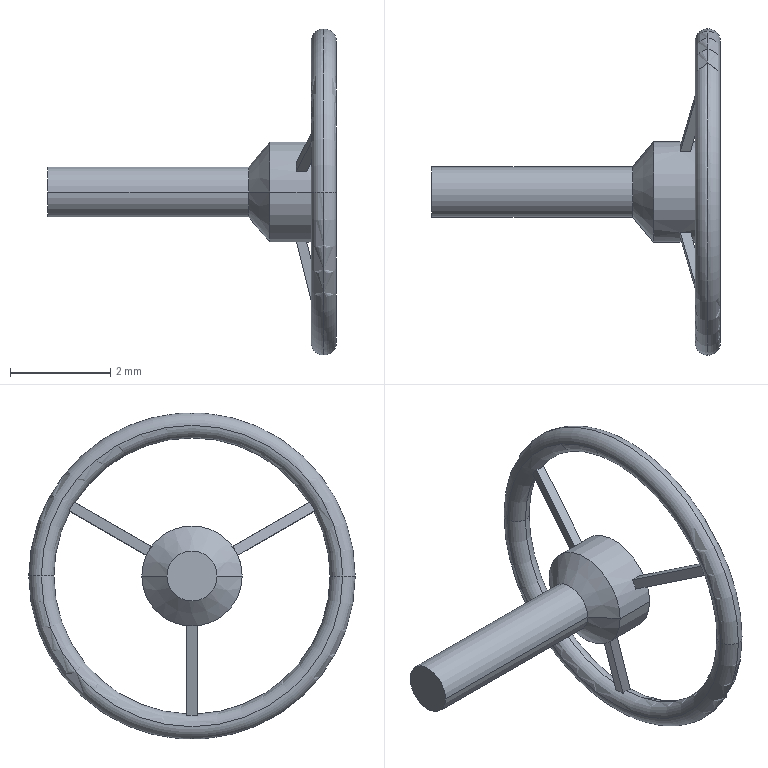Part | SolidWorks | features ICE 2, CirPattern 1, Fillet 1, Revolution 1 | 1 solid | 35 faces | box 5.75 x 6.5 x 6.5 mm | volume 10.173 mm3 | plane 19 | torus 8 | cylinder 4 | cone 4 | commonest cylinder face diameters 1 x2 2 x2
STEP:
#1=CARTESIAN_POINT('',(5.75,3.,0.));
#2=VERTEX_POINT('',#1);
#3=CARTESIAN_POINT('',(5.75,-3.,0.));
#4=VERTEX_POINT('',#3);
#5=CARTESIAN_POINT('',(5.75,0.,0.));
#6=DIRECTION('',(1.,0.,0.));
#7=DIRECTION('',(0.,-1.,0.));
#8=AXIS2_PLACEMENT_3D('',#5,#6,#7);
#9=CIRCLE('',#8,3.);
#10=EDGE_CURVE('',#2,#4,#9,.T.);
#11=ORIENTED_EDGE('',*,*,#10,.F.);
#12=CARTESIAN_POINT('',(5.5,3.25,0.));
#13=VERTEX_POINT('',#12);
#14=CARTESIAN_POINT('',(5.5,3.,0.));
#15=DIRECTION('',(0.,0.,1.));
#16=DIRECTION('',(0.,-1.,0.));
#17=AXIS2_PLACEMENT_3D('',#14,#15,#16);
#18=CIRCLE('',#17,0.25);
#19=EDGE_CURVE('',#2,#13,#18,.T.);
#20=ORIENTED_EDGE('',*,*,#19,.T.);
#21=CARTESIAN_POINT('',(5.5,-3.25,0.));
#22=VERTEX_POINT('',#21);
#23=CARTESIAN_POINT('',(5.5,0.,0.));
#24=DIRECTION('',(1.,0.,0.));
#25=DIRECTION('',(0.,-1.,0.));
#26=AXIS2_PLACEMENT_3D('',#23,#24,#25);
#27=CIRCLE('',#26,3.25);
#28=EDGE_CURVE('',#13,#22,#27,.T.);
#29=ORIENTED_EDGE('',*,*,#28,.T.);
#30=CARTESIAN_POINT('',(5.5,-3.,0.));
#31=DIRECTION('',(0.,0.,-1.));
#32=DIRECTION('',(-1.,0.,0.));
#33=AXIS2_PLACEMENT_3D('',#30,#31,#32);
#34=CIRCLE('',#33,0.25);
#35=EDGE_CURVE('',#4,#22,#34,.T.);
#36=ORIENTED_EDGE('',*,*,#35,.F.);
#37=EDGE_LOOP('',(#11,#20,#29,#36));
#38=FACE_OUTER_BOUND('',#37,.T.);
#39=CARTESIAN_POINT('',(5.5,0.,0.));
#40=DIRECTION('',(-1.,0.,0.));
#41=DIRECTION('',(0.,-1.,0.));
#42=AXIS2_PLACEMENT_3D('',#39,#40,#41);
#43=TOROIDAL_SURFACE('',#42,3.,0.25);
#44=ADVANCED_FACE('',(#38),#43,.T.);
#45=ORIENTED_EDGE('',*,*,#28,.F.);
#46=CARTESIAN_POINT('',(5.25,3.,0.));
#47=VERTEX_POINT('',#46);
#48=CARTESIAN_POINT('',(5.5,3.,0.));
#49=DIRECTION('',(0.,0.,1.));
#50=DIRECTION('',(0.,-1.,0.));
#51=AXIS2_PLACEMENT_3D('',#48,#49,#50);
#52=CIRCLE('',#51,0.25);
#53=EDGE_CURVE('',#13,#47,#52,.T.);
#54=ORIENTED_EDGE('',*,*,#53,.T.);
#55=CARTESIAN_POINT('',(5.25,-3.,0.));
#56=VERTEX_POINT('',#55);
#57=CARTESIAN_POINT('',(5.25,0.,0.));
#58=DIRECTION('',(-1.,0.,0.));
#59=DIRECTION('',(0.,-1.,0.));
#60=AXIS2_PLACEMENT_3D('',#57,#58,#59);
#61=CIRCLE('',#60,3.);
#62=EDGE_CURVE('',#56,#47,#61,.T.);
#63=ORIENTED_EDGE('',*,*,#62,.F.);
#64=CARTESIAN_POINT('',(5.5,-3.,0.));
#65=DIRECTION('',(0.,0.,-1.));
#66=DIRECTION('',(-1.,0.,0.));
#67=AXIS2_PLACEMENT_3D('',#64,#65,#66);
#68=CIRCLE('',#67,0.25);
#69=EDGE_CURVE('',#22,#56,#68,.T.);
#70=ORIENTED_EDGE('',*,*,#69,.F.);
#71=EDGE_LOOP('',(#45,#54,#63,#70));
#72=FACE_OUTER_BOUND('',#71,.T.);
#73=CARTESIAN_POINT('',(5.5,0.,0.));
#74=DIRECTION('',(-1.,0.,0.));
#75=DIRECTION('',(0.,-1.,0.));
#76=AXIS2_PLACEMENT_3D('',#73,#74,#75);
#77=TOROIDAL_SURFACE('',#76,3.,0.25);
#78=ADVANCED_FACE('',(#72),#77,.T.);
#79=CARTESIAN_POINT('',(4.,-0.5,0.));
#80=VERTEX_POINT('',#79);
#81=CARTESIAN_POINT('',(4.,0.5,0.));
#82=VERTEX_POINT('',#81);
#83=CARTESIAN_POINT('',(4.,0.,0.));
#84=DIRECTION('',(-1.,0.,0.));
#85=DIRECTION('',(0.,-1.,0.));
#86=AXIS2_PLACEMENT_3D('',#83,#84,#85);
#87=CIRCLE('',#86,0.5);
#88=EDGE_CURVE('',#80,#82,#87,.T.);
#89=ORIENTED_EDGE('',*,*,#88,.T.);
#90=CARTESIAN_POINT('',(0.,0.5,0.));
#91=VERTEX_POINT('',#90);
#92=CARTESIAN_POINT('',(0.,0.5,0.));
#93=DIRECTION('',(-1.,0.,0.));
#94=VECTOR('',#93,1000.);
#95=LINE('',#92,#94);
#96=EDGE_CURVE('',#82,#91,#95,.T.);
#97=ORIENTED_EDGE('',*,*,#96,.T.);
#98=CARTESIAN_POINT('',(0.,-0.5,0.));
#99=VERTEX_POINT('',#98);
#100=CARTESIAN_POINT('',(0.,0.,0.));
#101=DIRECTION('',(-1.,0.,0.));
#102=DIRECTION('',(0.,-1.,0.));
#103=AXIS2_PLACEMENT_3D('',#100,#101,#102);
#104=CIRCLE('',#103,0.5);
#105=EDGE_CURVE('',#99,#91,#104,.T.);
#106=ORIENTED_EDGE('',*,*,#105,.F.);
#107=CARTESIAN_POINT('',(0.,-0.5,0.));
#108=DIRECTION('',(-1.,0.,0.));
#109=VECTOR('',#108,1000.);
#110=LINE('',#107,#109);
#111=EDGE_CURVE('',#80,#99,#110,.T.);
#112=ORIENTED_EDGE('',*,*,#111,.F.);
#113=EDGE_LOOP('',(#89,#97,#106,#112));
#114=FACE_OUTER_BOUND('',#113,.T.);
#115=CARTESIAN_POINT('',(0.,0.,0.));
#116=DIRECTION('',(-1.,0.,0.));
#117=DIRECTION('',(0.,-1.,0.));
#118=AXIS2_PLACEMENT_3D('',#115,#116,#117);
#119=CYLINDRICAL_SURFACE('',#118,0.5);
#120=ADVANCED_FACE('',(#114),#119,.T.);
#121=ORIENTED_EDGE('',*,*,#88,.F.);
#122=CARTESIAN_POINT('',(4.42,-1.,0.));
#123=VERTEX_POINT('',#122);
#124=CARTESIAN_POINT('',(4.42,-1.,0.));
#125=DIRECTION('',(0.6428,-0.766,0.));
#126=VECTOR('',#125,1000.);
#127=LINE('',#124,#126);
#128=EDGE_CURVE('',#80,#123,#127,.T.);
#129=ORIENTED_EDGE('',*,*,#128,.T.);
#130=CARTESIAN_POINT('',(4.42,1.,0.));
#131=VERTEX_POINT('',#130);
#132=CARTESIAN_POINT('',(4.42,0.,0.));
#133=DIRECTION('',(-1.,0.,0.));
#134=DIRECTION('',(0.,-1.,0.));
#135=AXIS2_PLACEMENT_3D('',#132,#133,#134);
#136=CIRCLE('',#135,1.);
#137=EDGE_CURVE('',#123,#131,#136,.T.);
#138=ORIENTED_EDGE('',*,*,#137,.T.);
#139=CARTESIAN_POINT('',(4.42,1.,0.));
#140=DIRECTION('',(0.6428,0.766,0.));
#141=VECTOR('',#140,1000.);
#142=LINE('',#139,#141);
#143=EDGE_CURVE('',#82,#131,#142,.T.);
#144=ORIENTED_EDGE('',*,*,#143,.F.);
#145=EDGE_LOOP('',(#121,#129,#138,#144));
#146=FACE_OUTER_BOUND('',#145,.T.);
#147=CARTESIAN_POINT('',(4.42,0.,0.));
#148=DIRECTION('',(1.,0.,0.));
#149=DIRECTION('',(0.,1.,0.));
#150=AXIS2_PLACEMENT_3D('',#147,#148,#149);
#151=CONICAL_SURFACE('',#150,1.,0.8727);
#152=ADVANCED_FACE('',(#146),#151,.T.);
#153=CARTESIAN_POINT('',(4.997,0.,0.));
#154=VERTEX_POINT('',#153);
#155=CARTESIAN_POINT('',(5.25,1.,0.));
#156=VERTEX_POINT('',#155);
#157=CARTESIAN_POINT('',(4.997,0.,0.));
#158=DIRECTION('',(0.2449,0.9696,0.));
#159=VECTOR('',#158,1000.);
#160=LINE('',#157,#159);
#161=EDGE_CURVE('',#154,#156,#160,.T.);
#162=ORIENTED_EDGE('',*,*,#161,.F.);
#163=CARTESIAN_POINT('',(5.25,-1.,0.));
#164=VERTEX_POINT('',#163);
#165=CARTESIAN_POINT('',(4.997,0.,0.));
#166=DIRECTION('',(0.2449,-0.9696,0.));
#167=VECTOR('',#166,1000.);
#168=LINE('',#165,#167);
#169=EDGE_CURVE('',#154,#164,#168,.T.);
#170=ORIENTED_EDGE('',*,*,#169,.T.);
#171=CARTESIAN_POINT('',(5.25,0.,0.));
#172=DIRECTION('',(-1.,0.,0.));
#173=DIRECTION('',(0.,-1.,0.));
#174=AXIS2_PLACEMENT_3D('',#171,#172,#173);
#175=CIRCLE('',#174,1.);
#176=EDGE_CURVE('',#156,#164,#175,.T.);
#177=ORIENTED_EDGE('',*,*,#176,.F.);
#178=EDGE_LOOP('',(#162,#170,#177));
#179=FACE_OUTER_BOUND('',#178,.T.);
#180=CARTESIAN_POINT('',(1004.997,0.,0.));
#181=DIRECTION('',(1.,0.,0.));
#182=DIRECTION('',(0.,1.,0.));
#183=AXIS2_PLACEMENT_3D('',#180,#181,#182);
#184=CONICAL_SURFACE('',#183,3959.225,1.323);
#185=ADVANCED_FACE('',(#179),#184,.F.);
#186=ORIENTED_EDGE('',*,*,#62,.T.);
#187=CARTESIAN_POINT('',(5.5,2.75,0.));
#188=VERTEX_POINT('',#187);
#189=CARTESIAN_POINT('',(5.5,3.,0.));
#190=DIRECTION('',(0.,0.,1.));
#191=DIRECTION('',(0.,-1.,0.));
#192=AXIS2_PLACEMENT_3D('',#189,#190,#191);
#193=CIRCLE('',#192,0.25);
#194=EDGE_CURVE('',#47,#188,#193,.T.);
#195=ORIENTED_EDGE('',*,*,#194,.T.);
#196=CARTESIAN_POINT('',(5.5,2.43,1.287));
#197=VERTEX_POINT('',#196);
#198=CARTESIAN_POINT('',(5.5,0.,0.));
#199=DIRECTION('',(-1.,0.,0.));
#200=DIRECTION('',(0.,-1.,0.));
#201=AXIS2_PLACEMENT_3D('',#198,#199,#200);
#202=CIRCLE('',#201,2.75);
#203=EDGE_CURVE('',#197,#188,#202,.T.);
#204=ORIENTED_EDGE('',*,*,#203,.F.);
#205=CARTESIAN_POINT('',(5.4,2.448,1.298));
#206=VERTEX_POINT('',#205);
#207=CARTESIAN_POINT('',(5.4,2.448,1.298));
#208=CARTESIAN_POINT('',(5.432,2.436,1.291));
#209=CARTESIAN_POINT('',(5.466,2.43,1.287));
#210=CARTESIAN_POINT('',(5.5,2.43,1.287));
#211=B_SPLINE_CURVE_WITH_KNOTS('',3,(#207,#208,#209,#210),.UNSPECIFIED.,.F.,.F.,(4,4),(0.0003276,0.0004297),.UNSPECIFIED.);
#212=EDGE_CURVE('',#206,#197,#211,.T.);
#213=ORIENTED_EDGE('',*,*,#212,.F.);
#214=CARTESIAN_POINT('',(5.4,2.348,1.471));
#215=VERTEX_POINT('',#214);
#216=CARTESIAN_POINT('',(5.4,2.448,1.298));
#217=CARTESIAN_POINT('',(5.401,2.416,1.357));
#218=CARTESIAN_POINT('',(5.401,2.383,1.414));
#219=CARTESIAN_POINT('',(5.4,2.348,1.471));
#220=B_SPLINE_CURVE_WITH_KNOTS('',3,(#216,#217,#218,#219),.UNSPECIFIED.,.F.,.F.,(4,4),(0.0006048,0.0008047),.UNSPECIFIED.);
#221=EDGE_CURVE('',#206,#215,#220,.T.);
#222=ORIENTED_EDGE('',*,*,#221,.T.);
#223=CARTESIAN_POINT('',(5.5,2.33,1.461));
#224=VERTEX_POINT('',#223);
#225=CARTESIAN_POINT('',(5.4,2.348,1.471));
#226=CARTESIAN_POINT('',(5.432,2.336,1.464));
#227=CARTESIAN_POINT('',(5.466,2.33,1.461));
#228=CARTESIAN_POINT('',(5.5,2.33,1.461));
#229=B_SPLINE_CURVE_WITH_KNOTS('',3,(#225,#226,#227,#228),.UNSPECIFIED.,.F.,.F.,(4,4),(0.0003276,0.0004297),.UNSPECIFIED.);
#230=EDGE_CURVE('',#215,#224,#229,.T.);
#231=ORIENTED_EDGE('',*,*,#230,.T.);
#232=CARTESIAN_POINT('',(5.5,-2.33,1.461));
#233=VERTEX_POINT('',#232);
#234=CARTESIAN_POINT('',(5.5,0.,0.));
#235=DIRECTION('',(-1.,0.,0.));
#236=DIRECTION('',(0.,-1.,0.));
#237=AXIS2_PLACEMENT_3D('',#234,#235,#236);
#238=CIRCLE('',#237,2.75);
#239=EDGE_CURVE('',#233,#224,#238,.T.);
#240=ORIENTED_EDGE('',*,*,#239,.F.);
#241=CARTESIAN_POINT('',(5.4,-2.348,1.471));
#242=VERTEX_POINT('',#241);
#243=CARTESIAN_POINT('',(5.4,-2.348,1.471));
#244=CARTESIAN_POINT('',(5.432,-2.336,1.464));
#245=CARTESIAN_POINT('',(5.466,-2.33,1.461));
#246=CARTESIAN_POINT('',(5.5,-2.33,1.461));
#247=B_SPLINE_CURVE_WITH_KNOTS('',3,(#243,#244,#245,#246),.UNSPECIFIED.,.F.,.F.,(4,4),(0.0003276,0.0004297),.UNSPECIFIED.);
#248=EDGE_CURVE('',#242,#233,#247,.T.);
#249=ORIENTED_EDGE('',*,*,#248,.F.);
#250=CARTESIAN_POINT('',(5.4,-2.448,1.298));
#251=VERTEX_POINT('',#250);
#252=CARTESIAN_POINT('',(5.4,-2.348,1.471));
#253=CARTESIAN_POINT('',(5.401,-2.383,1.414));
#254=CARTESIAN_POINT('',(5.401,-2.416,1.357));
#255=CARTESIAN_POINT('',(5.4,-2.448,1.298));
#256=B_SPLINE_CURVE_WITH_KNOTS('',3,(#252,#253,#254,#255),.UNSPECIFIED.,.F.,.F.,(4,4),(0.0001603,0.0003603),.UNSPECIFIED.);
#257=EDGE_CURVE('',#242,#251,#256,.T.);
#258=ORIENTED_EDGE('',*,*,#257,.T.);
#259=CARTESIAN_POINT('',(5.5,-2.43,1.287));
#260=VERTEX_POINT('',#259);
#261=CARTESIAN_POINT('',(5.4,-2.448,1.298));
#262=CARTESIAN_POINT('',(5.432,-2.436,1.291));
#263=CARTESIAN_POINT('',(5.466,-2.43,1.287));
#264=CARTESIAN_POINT('',(5.5,-2.43,1.287));
#265=B_SPLINE_CURVE_WITH_KNOTS('',3,(#261,#262,#263,#264),.UNSPECIFIED.,.F.,.F.,(4,4),(0.0003276,0.0004297),.UNSPECIFIED.);
#266=EDGE_CURVE('',#251,#260,#265,.T.);
#267=ORIENTED_EDGE('',*,*,#266,.T.);
#268=CARTESIAN_POINT('',(5.5,-2.75,0.));
#269=VERTEX_POINT('',#268);
#270=CARTESIAN_POINT('',(5.5,0.,0.));
#271=DIRECTION('',(-1.,0.,0.));
#272=DIRECTION('',(0.,-1.,0.));
#273=AXIS2_PLACEMENT_3D('',#270,#271,#272);
#274=CIRCLE('',#273,2.75);
#275=EDGE_CURVE('',#269,#260,#274,.T.);
#276=ORIENTED_EDGE('',*,*,#275,.F.);
#277=CARTESIAN_POINT('',(5.5,-3.,0.));
#278=DIRECTION('',(0.,0.,-1.));
#279=DIRECTION('',(-1.,0.,0.));
#280=AXIS2_PLACEMENT_3D('',#277,#278,#279);
#281=CIRCLE('',#280,0.25);
#282=EDGE_CURVE('',#56,#269,#281,.T.);
#283=ORIENTED_EDGE('',*,*,#282,.F.);
#284=EDGE_LOOP('',(#186,#195,#204,#213,#222,#231,#240,#249,#258,#267,#276,#283));
#285=FACE_OUTER_BOUND('',#284,.T.);
#286=CARTESIAN_POINT('',(5.5,0.,0.));
#287=DIRECTION('',(-1.,0.,0.));
#288=DIRECTION('',(0.,-1.,0.));
#289=AXIS2_PLACEMENT_3D('',#286,#287,#288);
#290=TOROIDAL_SURFACE('',#289,3.,0.25);
#291=ADVANCED_FACE('',(#285),#290,.T.);
#292=ORIENTED_EDGE('',*,*,#203,.T.);
#293=CARTESIAN_POINT('',(5.5,3.,0.));
#294=DIRECTION('',(0.,0.,1.));
#295=DIRECTION('',(0.,-1.,0.));
#296=AXIS2_PLACEMENT_3D('',#293,#294,#295);
#297=CIRCLE('',#296,0.25);
#298=EDGE_CURVE('',#188,#2,#297,.T.);
#299=ORIENTED_EDGE('',*,*,#298,.T.);
#300=ORIENTED_EDGE('',*,*,#10,.T.);
#301=CARTESIAN_POINT('',(5.5,-3.,0.));
#302=DIRECTION('',(0.,0.,-1.));
#303=DIRECTION('',(-1.,0.,0.));
#304=AXIS2_PLACEMENT_3D('',#301,#302,#303);
#305=CIRCLE('',#304,0.25);
#306=EDGE_CURVE('',#269,#4,#305,.T.);
#307=ORIENTED_EDGE('',*,*,#306,.F.);
#308=ORIENTED_EDGE('',*,*,#275,.T.);
#309=CARTESIAN_POINT('',(5.608,-2.451,1.3));
#310=VERTEX_POINT('',#309);
#311=CARTESIAN_POINT('',(5.5,-2.43,1.287));
#312=CARTESIAN_POINT('',(5.537,-2.43,1.287));
#313=CARTESIAN_POINT('',(5.574,-2.437,1.292));
#314=CARTESIAN_POINT('',(5.608,-2.451,1.3));
#315=B_SPLINE_CURVE_WITH_KNOTS('',3,(#311,#312,#313,#314),.UNSPECIFIED.,.F.,.F.,(4,4),(0.000000197,0.000111),.UNSPECIFIED.);
#316=EDGE_CURVE('',#260,#310,#315,.T.);
#317=ORIENTED_EDGE('',*,*,#316,.T.);
#318=CARTESIAN_POINT('',(5.608,-2.351,1.473));
#319=VERTEX_POINT('',#318);
#320=CARTESIAN_POINT('',(5.608,-2.451,1.3));
#321=CARTESIAN_POINT('',(5.608,-2.42,1.359));
#322=CARTESIAN_POINT('',(5.608,-2.387,1.417));
#323=CARTESIAN_POINT('',(5.608,-2.351,1.473));
#324=B_SPLINE_CURVE_WITH_KNOTS('',3,(#320,#321,#322,#323),.UNSPECIFIED.,.F.,.F.,(4,4),(0.0006711,0.0008713),.UNSPECIFIED.);
#325=EDGE_CURVE('',#310,#319,#324,.T.);
#326=ORIENTED_EDGE('',*,*,#325,.T.);
#327=CARTESIAN_POINT('',(5.5,-2.33,1.461));
#328=CARTESIAN_POINT('',(5.537,-2.33,1.461));
#329=CARTESIAN_POINT('',(5.574,-2.337,1.465));
#330=CARTESIAN_POINT('',(5.608,-2.351,1.473));
#331=B_SPLINE_CURVE_WITH_KNOTS('',3,(#327,#328,#329,#330),.UNSPECIFIED.,.F.,.F.,(4,4),(0.000000197,0.000111),.UNSPECIFIED.);
#332=EDGE_CURVE('',#233,#319,#331,.T.);
#333=ORIENTED_EDGE('',*,*,#332,.F.);
#334=ORIENTED_EDGE('',*,*,#239,.T.);
#335=CARTESIAN_POINT('',(5.608,2.351,1.473));
#336=VERTEX_POINT('',#335);
#337=CARTESIAN_POINT('',(5.5,2.33,1.461));
#338=CARTESIAN_POINT('',(5.537,2.33,1.461));
#339=CARTESIAN_POINT('',(5.574,2.337,1.465));
#340=CARTESIAN_POINT('',(5.608,2.351,1.473));
#341=B_SPLINE_CURVE_WITH_KNOTS('',3,(#337,#338,#339,#340),.UNSPECIFIED.,.F.,.F.,(4,4),(0.000000197,0.000111),.UNSPECIFIED.);
#342=EDGE_CURVE('',#224,#336,#341,.T.);
#343=ORIENTED_EDGE('',*,*,#342,.T.);
#344=CARTESIAN_POINT('',(5.608,2.451,1.3));
#345=VERTEX_POINT('',#344);
#346=CARTESIAN_POINT('',(5.608,2.351,1.473));
#347=CARTESIAN_POINT('',(5.608,2.387,1.417));
#348=CARTESIAN_POINT('',(5.608,2.42,1.359));
#349=CARTESIAN_POINT('',(5.608,2.451,1.3));
#350=B_SPLINE_CURVE_WITH_KNOTS('',3,(#346,#347,#348,#349),.UNSPECIFIED.,.F.,.F.,(4,4),(0.0001595,0.0003595),.UNSPECIFIED.);
#351=EDGE_CURVE('',#336,#345,#350,.T.);
#352=ORIENTED_EDGE('',*,*,#351,.T.);
#353=CARTESIAN_POINT('',(5.5,2.43,1.287));
#354=CARTESIAN_POINT('',(5.537,2.43,1.287));
#355=CARTESIAN_POINT('',(5.574,2.437,1.292));
#356=CARTESIAN_POINT('',(5.608,2.451,1.3));
#357=B_SPLINE_CURVE_WITH_KNOTS('',3,(#353,#354,#355,#356),.UNSPECIFIED.,.F.,.F.,(4,4),(0.000000197,0.000111),.UNSPECIFIED.);
#358=EDGE_CURVE('',#197,#345,#357,.T.);
#359=ORIENTED_EDGE('',*,*,#358,.F.);
#360=EDGE_LOOP('',(#292,#299,#300,#307,#308,#317,#326,#333,#334,#343,#352,#359));
#361=FACE_OUTER_BOUND('',#360,.T.);
#362=CARTESIAN_POINT('',(5.5,0.,0.));
#363=DIRECTION('',(-1.,0.,0.));
#364=DIRECTION('',(0.,-1.,0.));
#365=AXIS2_PLACEMENT_3D('',#362,#363,#364);
#366=TOROIDAL_SURFACE('',#365,3.,0.25);
#367=ADVANCED_FACE('',(#361),#366,.T.);
#368=CARTESIAN_POINT('',(4.952,-0.9117,0.4109));
#369=VERTEX_POINT('',#368);
#370=CARTESIAN_POINT('',(5.154,-0.9117,0.4109));
#371=VERTEX_POINT('',#370);
#372=CARTESIAN_POINT('',(0.,-0.9117,0.4109));
#373=DIRECTION('',(1.,0.,0.));
#374=VECTOR('',#373,1000.);
#375=LINE('',#372,#374);
#376=EDGE_CURVE('',#369,#371,#375,.T.);
#377=ORIENTED_EDGE('',*,*,#376,.F.);
#378=CARTESIAN_POINT('',(4.952,-0.8117,0.5841));
#379=VERTEX_POINT('',#378);
#380=CARTESIAN_POINT('',(4.952,-0.8117,0.5841));
#381=CARTESIAN_POINT('',(4.954,-0.8508,0.5298));
#382=CARTESIAN_POINT('',(4.954,-0.8842,0.4719));
#383=CARTESIAN_POINT('',(4.952,-0.9117,0.4109));
#384=(BOUNDED_CURVE()B_SPLINE_CURVE(3,(#380,#381,#382,#383),.UNSPECIFIED.,.F.,.F.)B_SPLINE_CURVE_WITH_KNOTS((4,4),(3.041,3.242),.UNSPECIFIED.)CURVE()GEOMETRIC_REPRESENTATION_ITEM()RATIONAL_B_SPLINE_CURVE((1.,0.9967,0.9967,1.))REPRESENTATION_ITEM(''));
#385=EDGE_CURVE('',#379,#369,#384,.T.);
#386=ORIENTED_EDGE('',*,*,#385,.F.);
#387=CARTESIAN_POINT('',(5.154,-0.8117,0.5841));
#388=VERTEX_POINT('',#387);
#389=CARTESIAN_POINT('',(0.,-0.8117,0.5841));
#390=DIRECTION('',(1.,0.,0.));
#391=VECTOR('',#390,1000.);
#392=LINE('',#389,#391);
#393=EDGE_CURVE('',#379,#388,#392,.T.);
#394=ORIENTED_EDGE('',*,*,#393,.T.);
#395=CARTESIAN_POINT('',(5.16,-0.866,0.5));
#396=VERTEX_POINT('',#395);
#397=CARTESIAN_POINT('',(5.16,-0.866,0.5));
#398=CARTESIAN_POINT('',(5.16,-0.8493,0.5289));
#399=CARTESIAN_POINT('',(5.158,-0.8312,0.557));
#400=CARTESIAN_POINT('',(5.154,-0.8117,0.5841));
#401=(BOUNDED_CURVE()B_SPLINE_CURVE(3,(#397,#398,#399,#400),.UNSPECIFIED.,.F.,.F.)B_SPLINE_CURVE_WITH_KNOTS((4,4),(3.142,3.242),.UNSPECIFIED.)CURVE()GEOMETRIC_REPRESENTATION_ITEM()RATIONAL_B_SPLINE_CURVE((1.,0.9992,0.9992,1.))REPRESENTATION_ITEM(''));
#402=EDGE_CURVE('',#396,#388,#401,.T.);
#403=ORIENTED_EDGE('',*,*,#402,.F.);
#404=CARTESIAN_POINT('',(5.154,-0.9117,0.4109));
#405=CARTESIAN_POINT('',(5.158,-0.898,0.4413));
#406=CARTESIAN_POINT('',(5.16,-0.8827,0.4711));
#407=CARTESIAN_POINT('',(5.16,-0.866,0.5));
#408=(BOUNDED_CURVE()B_SPLINE_CURVE(3,(#404,#405,#406,#407),.UNSPECIFIED.,.F.,.F.)B_SPLINE_CURVE_WITH_KNOTS((4,4),(3.041,3.142),.UNSPECIFIED.)CURVE()GEOMETRIC_REPRESENTATION_ITEM()RATIONAL_B_SPLINE_CURVE((1.,0.9992,0.9992,1.))REPRESENTATION_ITEM(''));
#409=EDGE_CURVE('',#371,#396,#408,.T.);
#410=ORIENTED_EDGE('',*,*,#409,.F.);
#411=EDGE_LOOP('',(#377,#386,#394,#403,#410));
#412=FACE_BOUND('',#411,.T.);
#413=CARTESIAN_POINT('',(4.952,0.8117,0.5841));
#414=VERTEX_POINT('',#413);
#415=CARTESIAN_POINT('',(5.154,0.8117,0.5841));
#416=VERTEX_POINT('',#415);
#417=CARTESIAN_POINT('',(0.,0.8117,0.5841));
#418=DIRECTION('',(1.,0.,0.));
#419=VECTOR('',#418,1000.);
#420=LINE('',#417,#419);
#421=EDGE_CURVE('',#414,#416,#420,.T.);
#422=ORIENTED_EDGE('',*,*,#421,.F.);
#423=CARTESIAN_POINT('',(4.952,0.9117,0.4109));
#424=VERTEX_POINT('',#423);
#425=CARTESIAN_POINT('',(4.952,0.9117,0.4109));
#426=CARTESIAN_POINT('',(4.954,0.8842,0.4719));
#427=CARTESIAN_POINT('',(4.954,0.8508,0.5298));
#428=CARTESIAN_POINT('',(4.952,0.8117,0.5841));
#429=(BOUNDED_CURVE()B_SPLINE_CURVE(3,(#425,#426,#427,#428),.UNSPECIFIED.,.F.,.F.)B_SPLINE_CURVE_WITH_KNOTS((4,4),(3.041,3.242),.UNSPECIFIED.)CURVE()GEOMETRIC_REPRESENTATION_ITEM()RATIONAL_B_SPLINE_CURVE((1.,0.9967,0.9967,1.))REPRESENTATION_ITEM(''));
#430=EDGE_CURVE('',#424,#414,#429,.T.);
#431=ORIENTED_EDGE('',*,*,#430,.F.);
#432=CARTESIAN_POINT('',(5.154,0.9117,0.4109));
#433=VERTEX_POINT('',#432);
#434=CARTESIAN_POINT('',(0.,0.9117,0.4109));
#435=DIRECTION('',(1.,0.,0.));
#436=VECTOR('',#435,1000.);
#437=LINE('',#434,#436);
#438=EDGE_CURVE('',#424,#433,#437,.T.);
#439=ORIENTED_EDGE('',*,*,#438,.T.);
#440=CARTESIAN_POINT('',(5.16,0.866,0.5));
#441=VERTEX_POINT('',#440);
#442=CARTESIAN_POINT('',(5.16,0.866,0.5));
#443=CARTESIAN_POINT('',(5.16,0.8827,0.4711));
#444=CARTESIAN_POINT('',(5.158,0.898,0.4413));
#445=CARTESIAN_POINT('',(5.154,0.9117,0.4109));
#446=(BOUNDED_CURVE()B_SPLINE_CURVE(3,(#442,#443,#444,#445),.UNSPECIFIED.,.F.,.F.)B_SPLINE_CURVE_WITH_KNOTS((4,4),(3.142,3.242),.UNSPECIFIED.)CURVE()GEOMETRIC_REPRESENTATION_ITEM()RATIONAL_B_SPLINE_CURVE((1.,0.9992,0.9992,1.))REPRESENTATION_ITEM(''));
#447=EDGE_CURVE('',#441,#433,#446,.T.);
#448=ORIENTED_EDGE('',*,*,#447,.F.);
#449=CARTESIAN_POINT('',(5.154,0.8117,0.5841));
#450=CARTESIAN_POINT('',(5.158,0.8312,0.557));
#451=CARTESIAN_POINT('',(5.16,0.8493,0.5289));
#452=CARTESIAN_POINT('',(5.16,0.866,0.5));
#453=(BOUNDED_CURVE()B_SPLINE_CURVE(3,(#449,#450,#451,#452),.UNSPECIFIED.,.F.,.F.)B_SPLINE_CURVE_WITH_KNOTS((4,4),(3.041,3.142),.UNSPECIFIED.)CURVE()GEOMETRIC_REPRESENTATION_ITEM()RATIONAL_B_SPLINE_CURVE((1.,0.9992,0.9992,1.))REPRESENTATION_ITEM(''));
#454=EDGE_CURVE('',#416,#441,#453,.T.);
#455=ORIENTED_EDGE('',*,*,#454,.F.);
#456=EDGE_LOOP('',(#422,#431,#439,#448,#455));
#457=FACE_BOUND('',#456,.T.);
#458=CARTESIAN_POINT('',(5.25,0.,0.));
#459=DIRECTION('',(-1.,0.,0.));
#460=DIRECTION('',(0.,-1.,0.));
#461=AXIS2_PLACEMENT_3D('',#458,#459,#460);
#462=CIRCLE('',#461,1.);
#463=EDGE_CURVE('',#164,#156,#462,.T.);
#464=ORIENTED_EDGE('',*,*,#463,.T.);
#465=CARTESIAN_POINT('',(0.,1.,0.));
#466=DIRECTION('',(-1.,0.,0.));
#467=VECTOR('',#466,1000.);
#468=LINE('',#465,#467);
#469=EDGE_CURVE('',#156,#131,#468,.T.);
#470=ORIENTED_EDGE('',*,*,#469,.T.);
#471=ORIENTED_EDGE('',*,*,#137,.F.);
#472=CARTESIAN_POINT('',(0.,-1.,0.));
#473=DIRECTION('',(-1.,0.,0.));
#474=VECTOR('',#473,1000.);
#475=LINE('',#472,#474);
#476=EDGE_CURVE('',#164,#123,#475,.T.);
#477=ORIENTED_EDGE('',*,*,#476,.F.);
#478=EDGE_LOOP('',(#464,#470,#471,#477));
#479=FACE_OUTER_BOUND('',#478,.T.);
#480=CARTESIAN_POINT('',(0.,0.,0.));
#481=DIRECTION('',(-1.,0.,0.));
#482=DIRECTION('',(0.,-1.,0.));
#483=AXIS2_PLACEMENT_3D('',#480,#481,#482);
#484=CYLINDRICAL_SURFACE('',#483,1.);
#485=ADVANCED_FACE('',(#412,#457,#479),#484,.T.);
#486=ORIENTED_EDGE('',*,*,#469,.F.);
#487=ORIENTED_EDGE('',*,*,#176,.T.);
#488=ORIENTED_EDGE('',*,*,#476,.T.);
#489=CARTESIAN_POINT('',(4.42,0.,0.));
#490=DIRECTION('',(-1.,0.,0.));
#491=DIRECTION('',(0.,-1.,0.));
#492=AXIS2_PLACEMENT_3D('',#489,#490,#491);
#493=CIRCLE('',#492,1.);
#494=EDGE_CURVE('',#131,#123,#493,.T.);
#495=ORIENTED_EDGE('',*,*,#494,.F.);
#496=EDGE_LOOP('',(#486,#487,#488,#495));
#497=FACE_OUTER_BOUND('',#496,.T.);
#498=CARTESIAN_POINT('',(4.952,0.1,-0.995));
#499=VERTEX_POINT('',#498);
#500=CARTESIAN_POINT('',(5.154,0.1,-0.995));
#501=VERTEX_POINT('',#500);
#502=CARTESIAN_POINT('',(0.,0.1,-0.995));
#503=DIRECTION('',(1.,0.,0.));
#504=VECTOR('',#503,1000.);
#505=LINE('',#502,#504);
#506=EDGE_CURVE('',#499,#501,#505,.T.);
#507=ORIENTED_EDGE('',*,*,#506,.F.);
#508=CARTESIAN_POINT('',(4.952,-0.1,-0.995));
#509=VERTEX_POINT('',#508);
#510=CARTESIAN_POINT('',(4.952,-0.1,-0.995));
#511=CARTESIAN_POINT('',(4.954,-0.03345,-1.002));
#512=CARTESIAN_POINT('',(4.954,0.03345,-1.002));
#513=CARTESIAN_POINT('',(4.952,0.1,-0.995));
#514=(BOUNDED_CURVE()B_SPLINE_CURVE(3,(#510,#511,#512,#513),.UNSPECIFIED.,.F.,.F.)B_SPLINE_CURVE_WITH_KNOTS((4,4),(3.041,3.242),.UNSPECIFIED.)CURVE()GEOMETRIC_REPRESENTATION_ITEM()RATIONAL_B_SPLINE_CURVE((1.,0.9967,0.9967,1.))REPRESENTATION_ITEM(''));
#515=EDGE_CURVE('',#509,#499,#514,.T.);
#516=ORIENTED_EDGE('',*,*,#515,.F.);
#517=CARTESIAN_POINT('',(5.154,-0.1,-0.995));
#518=VERTEX_POINT('',#517);
#519=CARTESIAN_POINT('',(0.,-0.1,-0.995));
#520=DIRECTION('',(1.,0.,0.));
#521=VECTOR('',#520,1000.);
#522=LINE('',#519,#521);
#523=EDGE_CURVE('',#509,#518,#522,.T.);
#524=ORIENTED_EDGE('',*,*,#523,.T.);
#525=CARTESIAN_POINT('',(5.16,0.,-1.));
#526=VERTEX_POINT('',#525);
#527=CARTESIAN_POINT('',(5.16,0.,-1.));
#528=CARTESIAN_POINT('',(5.16,-0.0334,-1.));
#529=CARTESIAN_POINT('',(5.158,-0.06676,-0.9983));
#530=CARTESIAN_POINT('',(5.154,-0.1,-0.995));
#531=(BOUNDED_CURVE()B_SPLINE_CURVE(3,(#527,#528,#529,#530),.UNSPECIFIED.,.F.,.F.)B_SPLINE_CURVE_WITH_KNOTS((4,4),(3.142,3.242),.UNSPECIFIED.)CURVE()GEOMETRIC_REPRESENTATION_ITEM()RATIONAL_B_SPLINE_CURVE((1.,0.9992,0.9992,1.))REPRESENTATION_ITEM(''));
#532=EDGE_CURVE('',#526,#518,#531,.T.);
#533=ORIENTED_EDGE('',*,*,#532,.F.);
#534=CARTESIAN_POINT('',(5.154,0.1,-0.995));
#535=CARTESIAN_POINT('',(5.158,0.06676,-0.9983));
#536=CARTESIAN_POINT('',(5.16,0.0334,-1.));
#537=CARTESIAN_POINT('',(5.16,0.,-1.));
#538=(BOUNDED_CURVE()B_SPLINE_CURVE(3,(#534,#535,#536,#537),.UNSPECIFIED.,.F.,.F.)B_SPLINE_CURVE_WITH_KNOTS((4,4),(3.041,3.142),.UNSPECIFIED.)CURVE()GEOMETRIC_REPRESENTATION_ITEM()RATIONAL_B_SPLINE_CURVE((1.,0.9992,0.9992,1.))REPRESENTATION_ITEM(''));
#539=EDGE_CURVE('',#501,#526,#538,.T.);
#540=ORIENTED_EDGE('',*,*,#539,.F.);
#541=EDGE_LOOP('',(#507,#516,#524,#533,#540));
#542=FACE_BOUND('',#541,.T.);
#543=CARTESIAN_POINT('',(0.,0.,0.));
#544=DIRECTION('',(-1.,0.,0.));
#545=DIRECTION('',(0.,-1.,0.));
#546=AXIS2_PLACEMENT_3D('',#543,#544,#545);
#547=CYLINDRICAL_SURFACE('',#546,1.);
#548=ADVANCED_FACE('',(#497,#542),#547,.T.);
#549=ORIENTED_EDGE('',*,*,#298,.F.);
#550=CARTESIAN_POINT('',(5.5,0.1,-2.748));
#551=VERTEX_POINT('',#550);
#552=CARTESIAN_POINT('',(5.5,0.,0.));
#553=DIRECTION('',(-1.,0.,0.));
#554=DIRECTION('',(0.,-1.,0.));
#555=AXIS2_PLACEMENT_3D('',#552,#553,#554);
#556=CIRCLE('',#555,2.75);
#557=EDGE_CURVE('',#188,#551,#556,.T.);
#558=ORIENTED_EDGE('',*,*,#557,.T.);
#559=CARTESIAN_POINT('',(5.608,0.1,-2.773));
#560=VERTEX_POINT('',#559);
#561=CARTESIAN_POINT('',(5.608,0.1,-2.773));
#562=CARTESIAN_POINT('',(5.591,0.1,-2.765));
#563=CARTESIAN_POINT('',(5.573,0.1,-2.758));
#564=CARTESIAN_POINT('',(5.537,0.1,-2.75));
#565=CARTESIAN_POINT('',(5.519,0.1,-2.748));
#566=CARTESIAN_POINT('',(5.5,0.1,-2.748));
#567=B_SPLINE_CURVE_WITH_KNOTS('',3,(#561,#562,#563,#564,#565,#566),.UNSPECIFIED.,.F.,.F.,(4,2,4),(0.001562,0.001617,0.001672),.UNSPECIFIED.);
#568=EDGE_CURVE('',#560,#551,#567,.T.);
#569=ORIENTED_EDGE('',*,*,#568,.F.);
#570=CARTESIAN_POINT('',(5.608,-0.1,-2.773));
#571=VERTEX_POINT('',#570);
#572=CARTESIAN_POINT('',(5.608,-0.1,-2.773));
#573=CARTESIAN_POINT('',(5.608,-0.03339,-2.775));
#574=CARTESIAN_POINT('',(5.608,0.03339,-2.775));
#575=CARTESIAN_POINT('',(5.608,0.1,-2.773));
#576=B_SPLINE_CURVE_WITH_KNOTS('',3,(#572,#573,#574,#575),.UNSPECIFIED.,.F.,.F.,(4,4),(0.0000002,0.0002002),.UNSPECIFIED.);
#577=EDGE_CURVE('',#571,#560,#576,.T.);
#578=ORIENTED_EDGE('',*,*,#577,.F.);
#579=CARTESIAN_POINT('',(5.5,-0.1,-2.748));
#580=VERTEX_POINT('',#579);
#581=CARTESIAN_POINT('',(5.608,-0.1,-2.773));
#582=CARTESIAN_POINT('',(5.591,-0.1,-2.765));
#583=CARTESIAN_POINT('',(5.573,-0.1,-2.758));
#584=CARTESIAN_POINT('',(5.537,-0.1,-2.75));
#585=CARTESIAN_POINT('',(5.519,-0.1,-2.748));
#586=CARTESIAN_POINT('',(5.5,-0.1,-2.748));
#587=B_SPLINE_CURVE_WITH_KNOTS('',3,(#581,#582,#583,#584,#585,#586),.UNSPECIFIED.,.F.,.F.,(4,2,4),(0.001562,0.001617,0.001672),.UNSPECIFIED.);
#588=EDGE_CURVE('',#571,#580,#587,.T.);
#589=ORIENTED_EDGE('',*,*,#588,.T.);
#590=CARTESIAN_POINT('',(5.5,0.,0.));
#591=DIRECTION('',(-1.,0.,0.));
#592=DIRECTION('',(0.,-1.,0.));
#593=AXIS2_PLACEMENT_3D('',#590,#591,#592);
#594=CIRCLE('',#593,2.75);
#595=EDGE_CURVE('',#580,#269,#594,.T.);
#596=ORIENTED_EDGE('',*,*,#595,.T.);
#597=ORIENTED_EDGE('',*,*,#306,.T.);
#598=CARTESIAN_POINT('',(5.75,0.,0.));
#599=DIRECTION('',(1.,0.,0.));
#600=DIRECTION('',(0.,-1.,0.));
#601=AXIS2_PLACEMENT_3D('',#598,#599,#600);
#602=CIRCLE('',#601,3.);
#603=EDGE_CURVE('',#4,#2,#602,.T.);
#604=ORIENTED_EDGE('',*,*,#603,.T.);
#605=EDGE_LOOP('',(#549,#558,#569,#578,#589,#596,#597,#604));
#606=FACE_OUTER_BOUND('',#605,.T.);
#607=CARTESIAN_POINT('',(5.5,0.,0.));
#608=DIRECTION('',(-1.,0.,0.));
#609=DIRECTION('',(0.,-1.,0.));
#610=AXIS2_PLACEMENT_3D('',#607,#608,#609);
#611=TOROIDAL_SURFACE('',#610,3.,0.25);
#612=ADVANCED_FACE('',(#606),#611,.T.);
#613=ORIENTED_EDGE('',*,*,#194,.F.);
#614=CARTESIAN_POINT('',(5.25,0.,0.));
#615=DIRECTION('',(-1.,0.,0.));
#616=DIRECTION('',(0.,-1.,0.));
#617=AXIS2_PLACEMENT_3D('',#614,#615,#616);
#618=CIRCLE('',#617,3.);
#619=EDGE_CURVE('',#47,#56,#618,.T.);
#620=ORIENTED_EDGE('',*,*,#619,.T.);
#621=ORIENTED_EDGE('',*,*,#282,.T.);
#622=ORIENTED_EDGE('',*,*,#595,.F.);
#623=CARTESIAN_POINT('',(5.4,-0.1,-2.769));
#624=VERTEX_POINT('',#623);
#625=CARTESIAN_POINT('',(5.5,-0.1,-2.748));
#626=CARTESIAN_POINT('',(5.483,-0.1,-2.748));
#627=CARTESIAN_POINT('',(5.466,-0.1,-2.75));
#628=CARTESIAN_POINT('',(5.433,-0.1,-2.757));
#629=CARTESIAN_POINT('',(5.416,-0.1,-2.762));
#630=CARTESIAN_POINT('',(5.4,-0.1,-2.769));
#631=B_SPLINE_CURVE_WITH_KNOTS('',3,(#625,#626,#627,#628,#629,#630),.UNSPECIFIED.,.F.,.F.,(4,2,4),(0.001251,0.001302,0.001353),.UNSPECIFIED.);
#632=EDGE_CURVE('',#580,#624,#631,.T.);
#633=ORIENTED_EDGE('',*,*,#632,.T.);
#634=CARTESIAN_POINT('',(5.4,0.1,-2.769));
#635=VERTEX_POINT('',#634);
#636=CARTESIAN_POINT('',(5.4,0.1,-2.769));
#637=CARTESIAN_POINT('',(5.401,0.03337,-2.771));
#638=CARTESIAN_POINT('',(5.401,-0.03337,-2.771));
#639=CARTESIAN_POINT('',(5.4,-0.1,-2.769));
#640=B_SPLINE_CURVE_WITH_KNOTS('',3,(#636,#637,#638,#639),.UNSPECIFIED.,.F.,.F.,(4,4),(0.0000002,0.0002002),.UNSPECIFIED.);
#641=EDGE_CURVE('',#635,#624,#640,.T.);
#642=ORIENTED_EDGE('',*,*,#641,.F.);
#643=CARTESIAN_POINT('',(5.5,0.1,-2.748));
#644=CARTESIAN_POINT('',(5.483,0.1,-2.748));
#645=CARTESIAN_POINT('',(5.466,0.1,-2.75));
#646=CARTESIAN_POINT('',(5.433,0.1,-2.757));
#647=CARTESIAN_POINT('',(5.416,0.1,-2.762));
#648=CARTESIAN_POINT('',(5.4,0.1,-2.769));
#649=B_SPLINE_CURVE_WITH_KNOTS('',3,(#643,#644,#645,#646,#647,#648),.UNSPECIFIED.,.F.,.F.,(4,2,4),(0.001251,0.001302,0.001353),.UNSPECIFIED.);
#650=EDGE_CURVE('',#551,#635,#649,.T.);
#651=ORIENTED_EDGE('',*,*,#650,.F.);
#652=ORIENTED_EDGE('',*,*,#557,.F.);
#653=EDGE_LOOP('',(#613,#620,#621,#622,#633,#642,#651,#652));
#654=FACE_OUTER_BOUND('',#653,.T.);
#655=CARTESIAN_POINT('',(5.5,0.,0.));
#656=DIRECTION('',(-1.,0.,0.));
#657=DIRECTION('',(0.,-1.,0.));
#658=AXIS2_PLACEMENT_3D('',#655,#656,#657);
#659=TOROIDAL_SURFACE('',#658,3.,0.25);
#660=ADVANCED_FACE('',(#654),#659,.T.);
#661=ORIENTED_EDGE('',*,*,#169,.F.);
#662=ORIENTED_EDGE('',*,*,#161,.T.);
#663=ORIENTED_EDGE('',*,*,#463,.F.);
#664=EDGE_LOOP('',(#661,#662,#663));
#665=FACE_OUTER_BOUND('',#664,.T.);
#666=CARTESIAN_POINT('',(1004.997,0.,0.));
#667=DIRECTION('',(1.,0.,0.));
#668=DIRECTION('',(0.,1.,0.));
#669=AXIS2_PLACEMENT_3D('',#666,#667,#668);
#670=CONICAL_SURFACE('',#669,3959.225,1.323);
#671=ADVANCED_FACE('',(#665),#670,.F.);
#672=ORIENTED_EDGE('',*,*,#128,.F.);
#673=CARTESIAN_POINT('',(4.,0.,0.));
#674=DIRECTION('',(-1.,0.,0.));
#675=DIRECTION('',(0.,-1.,0.));
#676=AXIS2_PLACEMENT_3D('',#673,#674,#675);
#677=CIRCLE('',#676,0.5);
#678=EDGE_CURVE('',#82,#80,#677,.T.);
#679=ORIENTED_EDGE('',*,*,#678,.F.);
#680=ORIENTED_EDGE('',*,*,#143,.T.);
#681=ORIENTED_EDGE('',*,*,#494,.T.);
#682=EDGE_LOOP('',(#672,#679,#680,#681));
#683=FACE_OUTER_BOUND('',#682,.T.);
#684=CARTESIAN_POINT('',(4.42,0.,0.));
#685=DIRECTION('',(1.,0.,0.));
#686=DIRECTION('',(0.,1.,0.));
#687=AXIS2_PLACEMENT_3D('',#684,#685,#686);
#688=CONICAL_SURFACE('',#687,1.,0.8727);
#689=ADVANCED_FACE('',(#683),#688,.T.);
#690=ORIENTED_EDGE('',*,*,#96,.F.);
#691=ORIENTED_EDGE('',*,*,#678,.T.);
#692=ORIENTED_EDGE('',*,*,#111,.T.);
#693=CARTESIAN_POINT('',(0.,0.,0.));
#694=DIRECTION('',(-1.,0.,0.));
#695=DIRECTION('',(0.,-1.,0.));
#696=AXIS2_PLACEMENT_3D('',#693,#694,#695);
#697=CIRCLE('',#696,0.5);
#698=EDGE_CURVE('',#91,#99,#697,.T.);
#699=ORIENTED_EDGE('',*,*,#698,.F.);
#700=EDGE_LOOP('',(#690,#691,#692,#699));
#701=FACE_OUTER_BOUND('',#700,.T.);
#702=CARTESIAN_POINT('',(0.,0.,0.));
#703=DIRECTION('',(-1.,0.,0.));
#704=DIRECTION('',(0.,-1.,0.));
#705=AXIS2_PLACEMENT_3D('',#702,#703,#704);
#706=CYLINDRICAL_SURFACE('',#705,0.5);
#707=ADVANCED_FACE('',(#701),#706,.T.);
#708=ORIENTED_EDGE('',*,*,#105,.T.);
#709=ORIENTED_EDGE('',*,*,#698,.T.);
#710=EDGE_LOOP('',(#708,#709));
#711=FACE_OUTER_BOUND('',#710,.T.);
#712=CARTESIAN_POINT('',(0.,0.,0.));
#713=DIRECTION('',(1.,0.,0.));
#714=DIRECTION('',(0.,1.,0.));
#715=AXIS2_PLACEMENT_3D('',#712,#713,#714);
#716=PLANE('',#715);
#717=ADVANCED_FACE('',(#711),#716,.F.);
#718=CARTESIAN_POINT('',(5.16,0.1,-1.));
#719=VERTEX_POINT('',#718);
#720=CARTESIAN_POINT('',(4.901,0.1,-0.7929));
#721=DIRECTION('',(0.7806,0.,-0.6251));
#722=VECTOR('',#721,1000.);
#723=LINE('',#720,#722);
#724=EDGE_CURVE('',#501,#719,#723,.T.);
#725=ORIENTED_EDGE('',*,*,#724,.F.);
#726=ORIENTED_EDGE('',*,*,#539,.T.);
#727=CARTESIAN_POINT('',(5.16,0.1,-1.));
#728=DIRECTION('',(0.,-1.,0.));
#729=VECTOR('',#728,1000.);
#730=LINE('',#727,#729);
#731=EDGE_CURVE('',#719,#526,#730,.T.);
#732=ORIENTED_EDGE('',*,*,#731,.F.);
#733=EDGE_LOOP('',(#725,#726,#732));
#734=FACE_OUTER_BOUND('',#733,.T.);
#735=CARTESIAN_POINT('',(4.901,0.1,-0.7929));
#736=DIRECTION('',(-0.6251,0.,-0.7806));
#737=DIRECTION('',(-0.7806,0.,0.6251));
#738=AXIS2_PLACEMENT_3D('',#735,#736,#737);
#739=PLANE('',#738);
#740=ADVANCED_FACE('',(#734),#739,.F.);
#741=ORIENTED_EDGE('',*,*,#568,.T.);
#742=ORIENTED_EDGE('',*,*,#650,.T.);
#743=CARTESIAN_POINT('',(4.901,0.1,-0.7929));
#744=DIRECTION('',(-0.2449,0.,0.9696));
#745=VECTOR('',#744,1000.);
#746=LINE('',#743,#745);
#747=EDGE_CURVE('',#635,#499,#746,.T.);
#748=ORIENTED_EDGE('',*,*,#747,.T.);
#749=ORIENTED_EDGE('',*,*,#506,.T.);
#750=ORIENTED_EDGE('',*,*,#724,.T.);
#751=CARTESIAN_POINT('',(5.16,0.1,-1.));
#752=DIRECTION('',(0.2449,0.,-0.9696));
#753=VECTOR('',#752,1000.);
#754=LINE('',#751,#753);
#755=EDGE_CURVE('',#719,#560,#754,.T.);
#756=ORIENTED_EDGE('',*,*,#755,.T.);
#757=EDGE_LOOP('',(#741,#742,#748,#749,#750,#756));
#758=FACE_OUTER_BOUND('',#757,.T.);
#759=CARTESIAN_POINT('',(0.,0.1,0.));
#760=DIRECTION('',(0.,-1.,0.));
#761=DIRECTION('',(0.,0.,-1.));
#762=AXIS2_PLACEMENT_3D('',#759,#760,#761);
#763=PLANE('',#762);
#764=ADVANCED_FACE('',(#758),#763,.F.);
#765=ORIENTED_EDGE('',*,*,#632,.F.);
#766=ORIENTED_EDGE('',*,*,#588,.F.);
#767=CARTESIAN_POINT('',(5.16,-0.1,-1.));
#768=VERTEX_POINT('',#767);
#769=CARTESIAN_POINT('',(5.16,-0.1,-1.));
#770=DIRECTION('',(0.2449,0.,-0.9696));
#771=VECTOR('',#770,1000.);
#772=LINE('',#769,#771);
#773=EDGE_CURVE('',#768,#571,#772,.T.);
#774=ORIENTED_EDGE('',*,*,#773,.F.);
#775=CARTESIAN_POINT('',(4.901,-0.1,-0.7929));
#776=DIRECTION('',(0.7806,0.,-0.6251));
#777=VECTOR('',#776,1000.);
#778=LINE('',#775,#777);
#779=EDGE_CURVE('',#518,#768,#778,.T.);
#780=ORIENTED_EDGE('',*,*,#779,.F.);
#781=ORIENTED_EDGE('',*,*,#523,.F.);
#782=CARTESIAN_POINT('',(4.901,-0.1,-0.7929));
#783=DIRECTION('',(-0.2449,0.,0.9696));
#784=VECTOR('',#783,1000.);
#785=LINE('',#782,#784);
#786=EDGE_CURVE('',#624,#509,#785,.T.);
#787=ORIENTED_EDGE('',*,*,#786,.F.);
#788=EDGE_LOOP('',(#765,#766,#774,#780,#781,#787));
#789=FACE_OUTER_BOUND('',#788,.T.);
#790=CARTESIAN_POINT('',(0.,-0.1,0.));
#791=DIRECTION('',(0.,-1.,0.));
#792=DIRECTION('',(0.,0.,-1.));
#793=AXIS2_PLACEMENT_3D('',#790,#791,#792);
#794=PLANE('',#793);
#795=ADVANCED_FACE('',(#789),#794,.T.);
#796=CARTESIAN_POINT('',(5.16,0.1,-1.));
#797=DIRECTION('',(0.,-1.,0.));
#798=VECTOR('',#797,1000.);
#799=LINE('',#796,#798);
#800=EDGE_CURVE('',#526,#768,#799,.T.);
#801=ORIENTED_EDGE('',*,*,#800,.F.);
#802=ORIENTED_EDGE('',*,*,#532,.T.);
#803=ORIENTED_EDGE('',*,*,#779,.T.);
#804=EDGE_LOOP('',(#801,#802,#803));
#805=FACE_OUTER_BOUND('',#804,.T.);
#806=CARTESIAN_POINT('',(4.901,0.1,-0.7929));
#807=DIRECTION('',(-0.6251,0.,-0.7806));
#808=DIRECTION('',(-0.7806,0.,0.6251));
#809=AXIS2_PLACEMENT_3D('',#806,#807,#808);
#810=PLANE('',#809);
#811=ADVANCED_FACE('',(#805),#810,.F.);
#812=ORIENTED_EDGE('',*,*,#773,.T.);
#813=ORIENTED_EDGE('',*,*,#577,.T.);
#814=ORIENTED_EDGE('',*,*,#755,.F.);
#815=ORIENTED_EDGE('',*,*,#731,.T.);
#816=ORIENTED_EDGE('',*,*,#800,.T.);
#817=EDGE_LOOP('',(#812,#813,#814,#815,#816));
#818=FACE_OUTER_BOUND('',#817,.T.);
#819=CARTESIAN_POINT('',(5.16,0.1,-1.));
#820=DIRECTION('',(-0.9696,0.,-0.2449));
#821=DIRECTION('',(-0.2449,0.,0.9696));
#822=AXIS2_PLACEMENT_3D('',#819,#820,#821);
#823=PLANE('',#822);
#824=ADVANCED_FACE('',(#818),#823,.F.);
#825=ORIENTED_EDGE('',*,*,#747,.F.);
#826=ORIENTED_EDGE('',*,*,#641,.T.);
#827=ORIENTED_EDGE('',*,*,#786,.T.);
#828=ORIENTED_EDGE('',*,*,#515,.T.);
#829=EDGE_LOOP('',(#825,#826,#827,#828));
#830=FACE_OUTER_BOUND('',#829,.T.);
#831=CARTESIAN_POINT('',(4.901,0.1,-0.7929));
#832=DIRECTION('',(0.9696,0.,0.2449));
#833=DIRECTION('',(0.2449,0.,-0.9696));
#834=AXIS2_PLACEMENT_3D('',#831,#832,#833);
#835=PLANE('',#834);
#836=ADVANCED_FACE('',(#830),#835,.F.);
#837=ORIENTED_EDGE('',*,*,#53,.F.);
#838=CARTESIAN_POINT('',(5.5,0.,0.));
#839=DIRECTION('',(1.,0.,0.));
#840=DIRECTION('',(0.,-1.,0.));
#841=AXIS2_PLACEMENT_3D('',#838,#839,#840);
#842=CIRCLE('',#841,3.25);
#843=EDGE_CURVE('',#22,#13,#842,.T.);
#844=ORIENTED_EDGE('',*,*,#843,.F.);
#845=ORIENTED_EDGE('',*,*,#69,.T.);
#846=ORIENTED_EDGE('',*,*,#619,.F.);
#847=EDGE_LOOP('',(#837,#844,#845,#846));
#848=FACE_OUTER_BOUND('',#847,.T.);
#849=CARTESIAN_POINT('',(5.5,0.,0.));
#850=DIRECTION('',(-1.,0.,0.));
#851=DIRECTION('',(0.,-1.,0.));
#852=AXIS2_PLACEMENT_3D('',#849,#850,#851);
#853=TOROIDAL_SURFACE('',#852,3.,0.25);
#854=ADVANCED_FACE('',(#848),#853,.T.);
#855=ORIENTED_EDGE('',*,*,#19,.F.);
#856=ORIENTED_EDGE('',*,*,#603,.F.);
#857=ORIENTED_EDGE('',*,*,#35,.T.);
#858=ORIENTED_EDGE('',*,*,#843,.T.);
#859=EDGE_LOOP('',(#855,#856,#857,#858));
#860=FACE_OUTER_BOUND('',#859,.T.);
#861=CARTESIAN_POINT('',(5.5,0.,0.));
#862=DIRECTION('',(-1.,0.,0.));
#863=DIRECTION('',(0.,-1.,0.));
#864=AXIS2_PLACEMENT_3D('',#861,#862,#863);
#865=TOROIDAL_SURFACE('',#864,3.,0.25);
#866=ADVANCED_FACE('',(#860),#865,.T.);
#867=CARTESIAN_POINT('',(5.16,0.816,0.5866));
#868=VERTEX_POINT('',#867);
#869=CARTESIAN_POINT('',(4.901,0.6367,0.4831));
#870=DIRECTION('',(0.7806,0.5413,0.3125));
#871=VECTOR('',#870,1000.);
#872=LINE('',#869,#871);
#873=EDGE_CURVE('',#416,#868,#872,.T.);
#874=ORIENTED_EDGE('',*,*,#873,.F.);
#875=ORIENTED_EDGE('',*,*,#454,.T.);
#876=CARTESIAN_POINT('',(5.16,0.816,0.5866));
#877=DIRECTION('',(0.,0.5,-0.866));
#878=VECTOR('',#877,1000.);
#879=LINE('',#876,#878);
#880=EDGE_CURVE('',#868,#441,#879,.T.);
#881=ORIENTED_EDGE('',*,*,#880,.F.);
#882=EDGE_LOOP('',(#874,#875,#881));
#883=FACE_OUTER_BOUND('',#882,.T.);
#884=CARTESIAN_POINT('',(4.901,0.6367,0.4831));
#885=DIRECTION('',(-0.6251,0.676,0.3903));
#886=DIRECTION('',(-0.7342,-0.6789,0.));
#887=AXIS2_PLACEMENT_3D('',#884,#885,#886);
#888=PLANE('',#887);
#889=ADVANCED_FACE('',(#883),#888,.F.);
#890=CARTESIAN_POINT('',(4.901,0.7367,0.3099));
#891=DIRECTION('',(-0.2449,-0.8397,-0.4848));
#892=VECTOR('',#891,1000.);
#893=LINE('',#890,#892);
#894=EDGE_CURVE('',#206,#424,#893,.T.);
#895=ORIENTED_EDGE('',*,*,#894,.T.);
#896=ORIENTED_EDGE('',*,*,#430,.T.);
#897=CARTESIAN_POINT('',(4.901,0.6367,0.4831));
#898=DIRECTION('',(-0.2449,-0.8397,-0.4848));
#899=VECTOR('',#898,1000.);
#900=LINE('',#897,#899);
#901=EDGE_CURVE('',#215,#414,#900,.T.);
#902=ORIENTED_EDGE('',*,*,#901,.F.);
#903=ORIENTED_EDGE('',*,*,#221,.F.);
#904=EDGE_LOOP('',(#895,#896,#902,#903));
#905=FACE_OUTER_BOUND('',#904,.T.);
#906=CARTESIAN_POINT('',(4.901,0.6367,0.4831));
#907=DIRECTION('',(0.9696,-0.2121,-0.1224));
#908=DIRECTION('',(0.2137,0.9769,0.));
#909=AXIS2_PLACEMENT_3D('',#906,#907,#908);
#910=PLANE('',#909);
#911=ADVANCED_FACE('',(#905),#910,.F.);
#912=ORIENTED_EDGE('',*,*,#901,.T.);
#913=ORIENTED_EDGE('',*,*,#421,.T.);
#914=ORIENTED_EDGE('',*,*,#873,.T.);
#915=CARTESIAN_POINT('',(5.16,0.816,0.5866));
#916=DIRECTION('',(0.2449,0.8397,0.4848));
#917=VECTOR('',#916,1000.);
#918=LINE('',#915,#917);
#919=EDGE_CURVE('',#868,#336,#918,.T.);
#920=ORIENTED_EDGE('',*,*,#919,.T.);
#921=ORIENTED_EDGE('',*,*,#342,.F.);
#922=ORIENTED_EDGE('',*,*,#230,.F.);
#923=EDGE_LOOP('',(#912,#913,#914,#920,#921,#922));
#924=FACE_OUTER_BOUND('',#923,.T.);
#925=CARTESIAN_POINT('',(0.,-0.05,0.0866));
#926=DIRECTION('',(0.,0.5,-0.866));
#927=DIRECTION('',(0.,0.866,0.5));
#928=AXIS2_PLACEMENT_3D('',#925,#926,#927);
#929=PLANE('',#928);
#930=ADVANCED_FACE('',(#924),#929,.F.);
#931=ORIENTED_EDGE('',*,*,#438,.F.);
#932=ORIENTED_EDGE('',*,*,#894,.F.);
#933=ORIENTED_EDGE('',*,*,#212,.T.);
#934=ORIENTED_EDGE('',*,*,#358,.T.);
#935=CARTESIAN_POINT('',(5.16,0.916,0.4134));
#936=VERTEX_POINT('',#935);
#937=CARTESIAN_POINT('',(5.16,0.916,0.4134));
#938=DIRECTION('',(0.2449,0.8397,0.4848));
#939=VECTOR('',#938,1000.);
#940=LINE('',#937,#939);
#941=EDGE_CURVE('',#936,#345,#940,.T.);
#942=ORIENTED_EDGE('',*,*,#941,.F.);
#943=CARTESIAN_POINT('',(4.901,0.7367,0.3099));
#944=DIRECTION('',(0.7806,0.5413,0.3125));
#945=VECTOR('',#944,1000.);
#946=LINE('',#943,#945);
#947=EDGE_CURVE('',#433,#936,#946,.T.);
#948=ORIENTED_EDGE('',*,*,#947,.F.);
#949=EDGE_LOOP('',(#931,#932,#933,#934,#942,#948));
#950=FACE_OUTER_BOUND('',#949,.T.);
#951=CARTESIAN_POINT('',(0.,0.05,-0.0866));
#952=DIRECTION('',(0.,0.5,-0.866));
#953=DIRECTION('',(0.,0.866,0.5));
#954=AXIS2_PLACEMENT_3D('',#951,#952,#953);
#955=PLANE('',#954);
#956=ADVANCED_FACE('',(#950),#955,.T.);
#957=CARTESIAN_POINT('',(5.16,0.816,0.5866));
#958=DIRECTION('',(0.,0.5,-0.866));
#959=VECTOR('',#958,1000.);
#960=LINE('',#957,#959);
#961=EDGE_CURVE('',#441,#936,#960,.T.);
#962=ORIENTED_EDGE('',*,*,#961,.F.);
#963=ORIENTED_EDGE('',*,*,#447,.T.);
#964=ORIENTED_EDGE('',*,*,#947,.T.);
#965=EDGE_LOOP('',(#962,#963,#964));
#966=FACE_OUTER_BOUND('',#965,.T.);
#967=CARTESIAN_POINT('',(4.901,0.6367,0.4831));
#968=DIRECTION('',(-0.6251,0.676,0.3903));
#969=DIRECTION('',(-0.7342,-0.6789,0.));
#970=AXIS2_PLACEMENT_3D('',#967,#968,#969);
#971=PLANE('',#970);
#972=ADVANCED_FACE('',(#966),#971,.F.);
#973=ORIENTED_EDGE('',*,*,#351,.F.);
#974=ORIENTED_EDGE('',*,*,#919,.F.);
#975=ORIENTED_EDGE('',*,*,#880,.T.);
#976=ORIENTED_EDGE('',*,*,#961,.T.);
#977=ORIENTED_EDGE('',*,*,#941,.T.);
#978=EDGE_LOOP('',(#973,#974,#975,#976,#977));
#979=FACE_OUTER_BOUND('',#978,.T.);
#980=CARTESIAN_POINT('',(5.16,0.816,0.5866));
#981=DIRECTION('',(-0.9696,0.2121,0.1224));
#982=DIRECTION('',(-0.2137,-0.9769,0.));
#983=AXIS2_PLACEMENT_3D('',#980,#981,#982);
#984=PLANE('',#983);
#985=ADVANCED_FACE('',(#979),#984,.F.);
#986=CARTESIAN_POINT('',(5.16,-0.916,0.4134));
#987=VERTEX_POINT('',#986);
#988=CARTESIAN_POINT('',(4.901,-0.7367,0.3099));
#989=DIRECTION('',(0.7806,-0.5413,0.3125));
#990=VECTOR('',#989,1000.);
#991=LINE('',#988,#990);
#992=EDGE_CURVE('',#371,#987,#991,.T.);
#993=ORIENTED_EDGE('',*,*,#992,.F.);
#994=ORIENTED_EDGE('',*,*,#409,.T.);
#995=CARTESIAN_POINT('',(5.16,-0.916,0.4134));
#996=DIRECTION('',(0.,0.5,0.866));
#997=VECTOR('',#996,1000.);
#998=LINE('',#995,#997);
#999=EDGE_CURVE('',#987,#396,#998,.T.);
#1000=ORIENTED_EDGE('',*,*,#999,.F.);
#1001=EDGE_LOOP('',(#993,#994,#1000));
#1002=FACE_OUTER_BOUND('',#1001,.T.);
#1003=CARTESIAN_POINT('',(4.901,-0.7367,0.3099));
#1004=DIRECTION('',(-0.6251,-0.676,0.3903));
#1005=DIRECTION('',(0.7342,-0.6789,0.));
#1006=AXIS2_PLACEMENT_3D('',#1003,#1004,#1005);
#1007=PLANE('',#1006);
#1008=ADVANCED_FACE('',(#1002),#1007,.F.);
#1009=CARTESIAN_POINT('',(4.901,-0.6367,0.4831));
#1010=DIRECTION('',(-0.2449,0.8397,-0.4848));
#1011=VECTOR('',#1010,1000.);
#1012=LINE('',#1009,#1011);
#1013=EDGE_CURVE('',#242,#379,#1012,.T.);
#1014=ORIENTED_EDGE('',*,*,#1013,.T.);
#1015=ORIENTED_EDGE('',*,*,#385,.T.);
#1016=CARTESIAN_POINT('',(4.901,-0.7367,0.3099));
#1017=DIRECTION('',(-0.2449,0.8397,-0.4848));
#1018=VECTOR('',#1017,1000.);
#1019=LINE('',#1016,#1018);
#1020=EDGE_CURVE('',#251,#369,#1019,.T.);
#1021=ORIENTED_EDGE('',*,*,#1020,.F.);
#1022=ORIENTED_EDGE('',*,*,#257,.F.);
#1023=EDGE_LOOP('',(#1014,#1015,#1021,#1022));
#1024=FACE_OUTER_BOUND('',#1023,.T.);
#1025=CARTESIAN_POINT('',(4.901,-0.7367,0.3099));
#1026=DIRECTION('',(0.9696,0.2121,-0.1224));
#1027=DIRECTION('',(-0.2137,0.9769,0.));
#1028=AXIS2_PLACEMENT_3D('',#1025,#1026,#1027);
#1029=PLANE('',#1028);
#1030=ADVANCED_FACE('',(#1024),#1029,.F.);
#1031=ORIENTED_EDGE('',*,*,#1020,.T.);
#1032=ORIENTED_EDGE('',*,*,#376,.T.);
#1033=ORIENTED_EDGE('',*,*,#992,.T.);
#1034=CARTESIAN_POINT('',(5.16,-0.916,0.4134));
#1035=DIRECTION('',(0.2449,-0.8397,0.4848));
#1036=VECTOR('',#1035,1000.);
#1037=LINE('',#1034,#1036);
#1038=EDGE_CURVE('',#987,#310,#1037,.T.);
#1039=ORIENTED_EDGE('',*,*,#1038,.T.);
#1040=ORIENTED_EDGE('',*,*,#316,.F.);
#1041=ORIENTED_EDGE('',*,*,#266,.F.);
#1042=EDGE_LOOP('',(#1031,#1032,#1033,#1039,#1040,#1041));
#1043=FACE_OUTER_BOUND('',#1042,.T.);
#1044=CARTESIAN_POINT('',(0.,-0.05,-0.0866));
#1045=DIRECTION('',(0.,0.5,0.866));
#1046=DIRECTION('',(0.,-0.866,0.5));
#1047=AXIS2_PLACEMENT_3D('',#1044,#1045,#1046);
#1048=PLANE('',#1047);
#1049=ADVANCED_FACE('',(#1043),#1048,.F.);
#1050=ORIENTED_EDGE('',*,*,#393,.F.);
#1051=ORIENTED_EDGE('',*,*,#1013,.F.);
#1052=ORIENTED_EDGE('',*,*,#248,.T.);
#1053=ORIENTED_EDGE('',*,*,#332,.T.);
#1054=CARTESIAN_POINT('',(5.16,-0.816,0.5866));
#1055=VERTEX_POINT('',#1054);
#1056=CARTESIAN_POINT('',(5.16,-0.816,0.5866));
#1057=DIRECTION('',(0.2449,-0.8397,0.4848));
#1058=VECTOR('',#1057,1000.);
#1059=LINE('',#1056,#1058);
#1060=EDGE_CURVE('',#1055,#319,#1059,.T.);
#1061=ORIENTED_EDGE('',*,*,#1060,.F.);
#1062=CARTESIAN_POINT('',(4.901,-0.6367,0.4831));
#1063=DIRECTION('',(0.7806,-0.5413,0.3125));
#1064=VECTOR('',#1063,1000.);
#1065=LINE('',#1062,#1064);
#1066=EDGE_CURVE('',#388,#1055,#1065,.T.);
#1067=ORIENTED_EDGE('',*,*,#1066,.F.);
#1068=EDGE_LOOP('',(#1050,#1051,#1052,#1053,#1061,#1067));
#1069=FACE_OUTER_BOUND('',#1068,.T.);
#1070=CARTESIAN_POINT('',(0.,0.05,0.0866));
#1071=DIRECTION('',(0.,0.5,0.866));
#1072=DIRECTION('',(0.,-0.866,0.5));
#1073=AXIS2_PLACEMENT_3D('',#1070,#1071,#1072);
#1074=PLANE('',#1073);
#1075=ADVANCED_FACE('',(#1069),#1074,.T.);
#1076=CARTESIAN_POINT('',(5.16,-0.916,0.4134));
#1077=DIRECTION('',(0.,0.5,0.866));
#1078=VECTOR('',#1077,1000.);
#1079=LINE('',#1076,#1078);
#1080=EDGE_CURVE('',#396,#1055,#1079,.T.);
#1081=ORIENTED_EDGE('',*,*,#1080,.F.);
#1082=ORIENTED_EDGE('',*,*,#402,.T.);
#1083=ORIENTED_EDGE('',*,*,#1066,.T.);
#1084=EDGE_LOOP('',(#1081,#1082,#1083));
#1085=FACE_OUTER_BOUND('',#1084,.T.);
#1086=CARTESIAN_POINT('',(4.901,-0.7367,0.3099));
#1087=DIRECTION('',(-0.6251,-0.676,0.3903));
#1088=DIRECTION('',(0.7342,-0.6789,0.));
#1089=AXIS2_PLACEMENT_3D('',#1086,#1087,#1088);
#1090=PLANE('',#1089);
#1091=ADVANCED_FACE('',(#1085),#1090,.F.);
#1092=ORIENTED_EDGE('',*,*,#325,.F.);
#1093=ORIENTED_EDGE('',*,*,#1038,.F.);
#1094=ORIENTED_EDGE('',*,*,#999,.T.);
#1095=ORIENTED_EDGE('',*,*,#1080,.T.);
#1096=ORIENTED_EDGE('',*,*,#1060,.T.);
#1097=EDGE_LOOP('',(#1092,#1093,#1094,#1095,#1096));
#1098=FACE_OUTER_BOUND('',#1097,.T.);
#1099=CARTESIAN_POINT('',(5.16,-0.916,0.4134));
#1100=DIRECTION('',(-0.9696,-0.2121,0.1224));
#1101=DIRECTION('',(0.2137,-0.9769,0.));
#1102=AXIS2_PLACEMENT_3D('',#1099,#1100,#1101);
#1103=PLANE('',#1102);
#1104=ADVANCED_FACE('',(#1098),#1103,.F.);
#1105=CLOSED_SHELL('',(#44,#78,#120,#152,#185,#291,#367,#485,#548,#612,#660,#671,#689,#707,#717,#740,#764,#795,#811,#824,#836,#854,#866,#889,#911,#930,#956,#972,#985,#1008,#1030,#1049,#1075,#1091,#1104));
#1106=MANIFOLD_SOLID_BREP('',#1105);
#1107=CARTESIAN_POINT('',(0.,0.,0.));
#1108=DIRECTION('',(0.,0.,1.));
#1109=DIRECTION('',(1.,0.,0.));
#1110=AXIS2_PLACEMENT_3D('',#1107,#1108,#1109);
#1111=(LENGTH_UNIT()NAMED_UNIT(*)SI_UNIT(.MILLI.,.METRE.));
#1112=UNCERTAINTY_MEASURE_WITH_UNIT(LENGTH_MEASURE(0.00001),#1111,'','');
#1113=(NAMED_UNIT(*)PLANE_ANGLE_UNIT()SI_UNIT($,.RADIAN.));
#1114=(NAMED_UNIT(*)SI_UNIT($,.STERADIAN.)SOLID_ANGLE_UNIT());
#1115=(GEOMETRIC_REPRESENTATION_CONTEXT(3)GLOBAL_UNCERTAINTY_ASSIGNED_CONTEXT((#1112))GLOBAL_UNIT_ASSIGNED_CONTEXT((#1111,#1113,#1114))REPRESENTATION_CONTEXT('',''));
#1116=ADVANCED_BREP_SHAPE_REPRESENTATION('',(#1106,#1110),#1115);